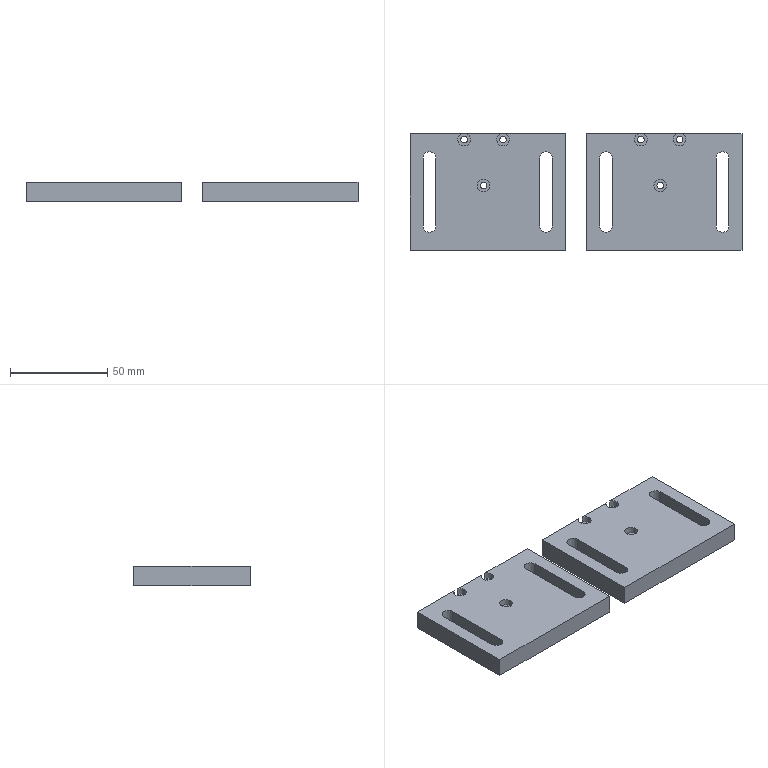CAM job | NX | 3-axis milling, drilling | part box 171 x 60 x 10 mm | stock box 176 x 65 x 12 mm
Tools:
number,name,description,diameter,corner_radius,flute_length,length,flutes
4,D4,平底铣刀-粗,4.0,0.0,25.0,75.0,2
9,D10,平底铣刀-粗,10.0,0.0,35.0,75.0,2
11,D4-J,平底铣刀-精,4.0,0.0,50.0,75.0,2
10,D10-J,平底铣刀-精,10.0,0.0,35.0,75.0,2
1,D80R0.8飞刀,圆鼻刀-粗,80.0,0.8,50.0,75.0,2
1,D80R0.8飞刀-J,圆鼻刀-精,80.0,0.8,50.0,75.0,2
2,D6倒角刀,倒角刀,6.0,0.0,3.0,25.0,2
13,ZT3.4,钻头,3.4,0.0,35.0,50.0,2
Operations:
program,operation,operation_type,tool,method,geometry_group,spindle_rpm,surface_speed,feed_per_tooth,feed_cut,feed_plunge,cut_length_mm,path_length_mm,cut_time_min,machine_time_min
B,底壁铣飞面一刀开粗_COPY,VolumeBased25DMillingOperation,D80R0.8飞刀,分层开粗-切深K-步距G,W-B,2800.0,703.696,0.5357,3000.0,100.0,1116.776,1976.734,0.3723,0.4583
B,底壁铣飞面一刀精光_COPY,VolumeBased25DMillingOperation,D80R0.8飞刀-J,侧刃精光-切深K-步距G,W-B,4000.0,1005.28,0.125,1000.0,100.0,278.998,314.998,0.279,0.2826
B,钻倒角_1,Operation,D6倒角刀,METHOD,W-B,8000.0,150.796,0.0625,1000.0,0.0,30.0,278.306,0.03,0.0548
B,平面去毛刺6X45L_COPY,SurfaceContour,D6倒角刀,爬面_倒角-切深0-步距G,W-B,6500.0,122.519,0.1154,1500.0,100.0,981.77,1600.123,0.6545,0.7163
A,顶面,FaceMilling,D80R0.8飞刀,侧刃精光-切深K-步距G,W-A,4000.0,1005.31,0.125,1000.0,100.0,265.0,301.0,0.265,0.2686
A,外形粗_2,VolumeBased25DMillingOperation,D10,METHOD,W-A,8000.0,251.327,0.3125,5000.0,80.0,9364.353,9552.853,1.873,1.892
A,沉头孔打点-深0.8,Operation,D6倒角刀,NONE,W-A,8000.0,150.796,0.0312,500.0,90.0,10.8,229.143,0.0216,0.0434
A,沉头孔-钻孔0段,Operation,ZT3.4,NONE,W-A,2800.0,29.908,0.0179,100.0,90.0,84.129,375.8,0.8413,0.8705
A,通腰槽粗_1,VolumeBased25DMillingOperation,D4,METHOD,W-A,6000.0,75.398,0.1,1200.0,100.0,13288.882,13636.19,11.074,11.109
A,铣孔开粗D4_1,CylinderMilling,D4,NONE,W-A,8000.0,100.531,0.075,1200.0,100.0,629.118,1062.361,0.5243,0.5676
A,铣孔精光D4_1,CylinderMilling,D4-J,精光步距切深关,W-A,8000.0,100.531,0.0312,500.0,100.0,113.737,546.98,0.2275,0.2708
A,腰槽精_1,VolumeBased25DMillingOperation,D4-J,METHOD,W-A,6000.0,113.0,0.0417,500.0,100.0,640.658,1077.28,1.281,1.325
A,仅选体,SurfaceContour,D6倒角刀,METHOD,W-A,8000.0,150.796,0.1875,3000.0,100.0,1053.068,1843.866,0.351,0.4301
A,铣倒角_1,PlanarMilling,D6倒角刀,NONE,W-A,8000.0,150.796,0.0312,500.0,100.0,175.233,548.267,0.3505,0.3878
A,外形半精_2,VolumeBased25DMillingOperation,D10-J,METHOD,W-A,8000.0,251.327,0.0625,1000.0,100.0,640.903,699.903,0.6409,0.6468